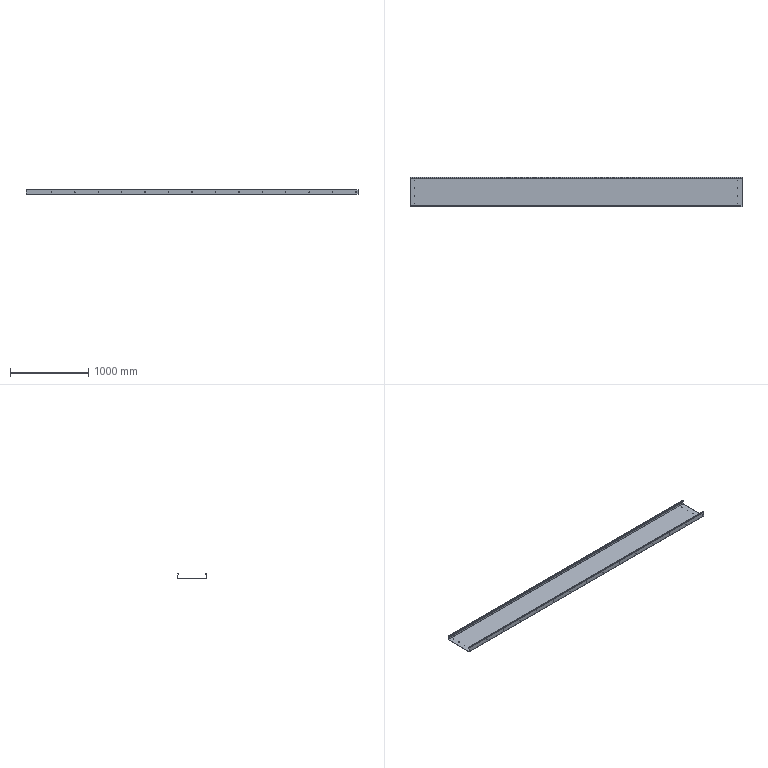Part | STEP file | TS-S89 | 1 solid | 126 faces | box 4250 x 380 x 62 mm | volume 4689334 mm3 | cylinder 84 | plane 42 | commonest cylinder face diameters 5.4 x56 7 x16 0.4 x6 4.4 x6